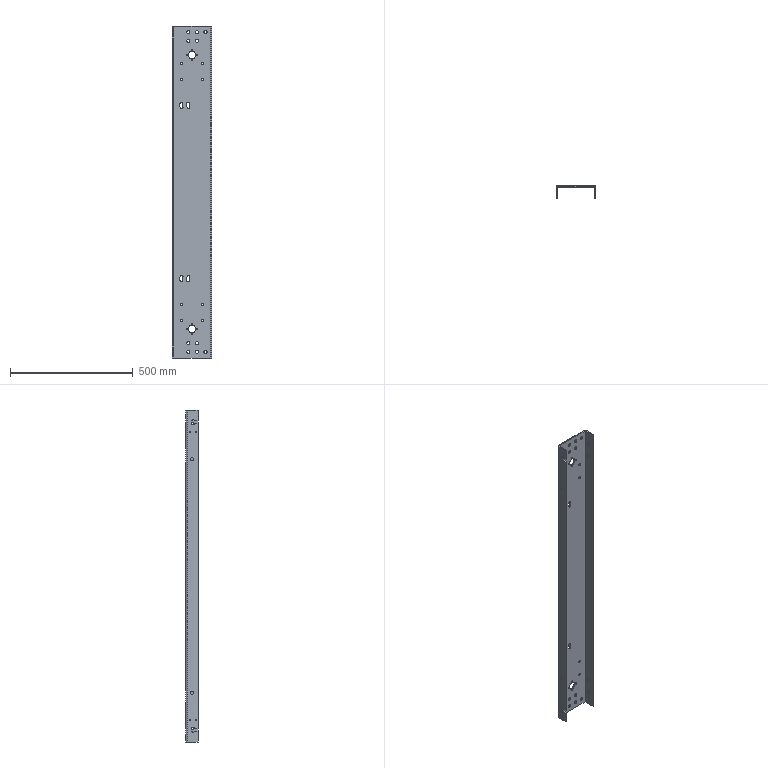Part | SolidWorks | features ICE 4, FlatPattern 1, SMBaseFlange 1, SheetMetal 1 | 1 solid | 130 faces | box 160 x 50 x 1350 mm | volume 1636068 mm3 | cylinder 96 | plane 34 | commonest cylinder face diameters 13 x32 6 x16 8.5 x16 12 x14 5 x8 11 x4